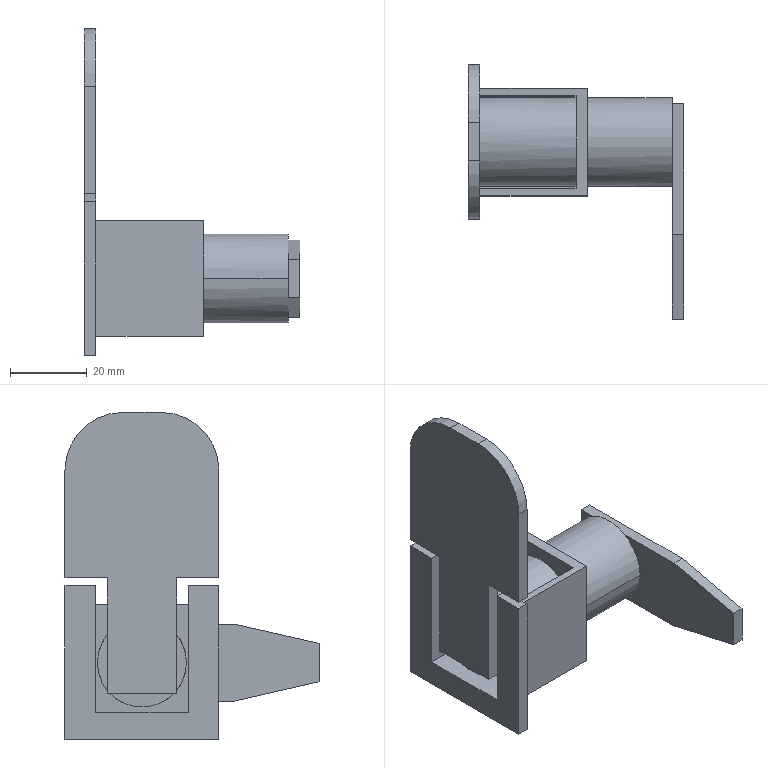Part | NX | features solid 2 | 1 solid | 50 faces | box 56 x 66 x 85 mm | volume 38408 mm3 | plane 44 | cylinder 6 | commonest cylinder face diameters 23.127 x4 30 x2
STEP:
#1=CARTESIAN_POINT('',(-1113.,-1266.5,497.5));
#2=VERTEX_POINT('',#1);
#3=CARTESIAN_POINT('',(-1113.,-1266.5,537.5));
#4=VERTEX_POINT('',#3);
#5=CARTESIAN_POINT('',(-1113.,-1266.5,497.5));
#6=DIRECTION('',(0.,0.,1.));
#7=VECTOR('',#6,1000.);
#8=LINE('',#5,#7);
#9=EDGE_CURVE('',#2,#4,#8,.T.);
#10=ORIENTED_EDGE('',*,*,#9,.T.);
#11=CARTESIAN_POINT('',(-1113.,-1258.5,537.5));
#12=VERTEX_POINT('',#11);
#13=CARTESIAN_POINT('',(-1113.,-1266.5,537.5));
#14=DIRECTION('',(0.,1.,0.));
#15=VECTOR('',#14,1000.);
#16=LINE('',#13,#15);
#17=EDGE_CURVE('',#4,#12,#16,.T.);
#18=ORIENTED_EDGE('',*,*,#17,.T.);
#19=CARTESIAN_POINT('',(-1113.,-1258.5,504.5));
#20=VERTEX_POINT('',#19);
#21=CARTESIAN_POINT('',(-1113.,-1258.5,537.5));
#22=DIRECTION('',(0.,0.,-1.));
#23=VECTOR('',#22,1000.);
#24=LINE('',#21,#23);
#25=EDGE_CURVE('',#12,#20,#24,.T.);
#26=ORIENTED_EDGE('',*,*,#25,.T.);
#27=CARTESIAN_POINT('',(-1113.,-1234.5,504.5));
#28=VERTEX_POINT('',#27);
#29=CARTESIAN_POINT('',(-1113.,-1258.5,504.5));
#30=DIRECTION('',(0.,1.,0.));
#31=VECTOR('',#30,1000.);
#32=LINE('',#29,#31);
#33=EDGE_CURVE('',#20,#28,#32,.T.);
#34=ORIENTED_EDGE('',*,*,#33,.T.);
#35=CARTESIAN_POINT('',(-1113.,-1234.5,537.5));
#36=VERTEX_POINT('',#35);
#37=CARTESIAN_POINT('',(-1113.,-1234.5,504.5));
#38=DIRECTION('',(0.,0.,1.));
#39=VECTOR('',#38,1000.);
#40=LINE('',#37,#39);
#41=EDGE_CURVE('',#28,#36,#40,.T.);
#42=ORIENTED_EDGE('',*,*,#41,.T.);
#43=CARTESIAN_POINT('',(-1113.,-1226.5,537.5));
#44=VERTEX_POINT('',#43);
#45=CARTESIAN_POINT('',(-1113.,-1234.5,537.5));
#46=DIRECTION('',(0.,1.,0.));
#47=VECTOR('',#46,1000.);
#48=LINE('',#45,#47);
#49=EDGE_CURVE('',#36,#44,#48,.T.);
#50=ORIENTED_EDGE('',*,*,#49,.T.);
#51=CARTESIAN_POINT('',(-1113.,-1226.5,497.5));
#52=VERTEX_POINT('',#51);
#53=CARTESIAN_POINT('',(-1113.,-1226.5,537.5));
#54=DIRECTION('',(0.,0.,-1.));
#55=VECTOR('',#54,1000.);
#56=LINE('',#53,#55);
#57=EDGE_CURVE('',#44,#52,#56,.T.);
#58=ORIENTED_EDGE('',*,*,#57,.T.);
#59=CARTESIAN_POINT('',(-1113.,-1226.5,497.5));
#60=DIRECTION('',(0.,-1.,0.));
#61=VECTOR('',#60,1000.);
#62=LINE('',#59,#61);
#63=EDGE_CURVE('',#52,#2,#62,.T.);
#64=ORIENTED_EDGE('',*,*,#63,.T.);
#65=EDGE_LOOP('',(#10,#18,#26,#34,#42,#50,#58,#64));
#66=FACE_BOUND('',#65,.T.);
#67=CARTESIAN_POINT('',(-1113.,-1266.5,537.5));
#68=DIRECTION('',(-1.,0.,0.));
#69=DIRECTION('',(0.,1.,0.));
#70=AXIS2_PLACEMENT_3D('',#67,#68,#69);
#71=PLANE('',#70);
#72=ADVANCED_FACE('',(#66),#71,.T.);
#73=CARTESIAN_POINT('',(-1110.,-1226.5,497.5));
#74=VERTEX_POINT('',#73);
#75=CARTESIAN_POINT('',(-1110.,-1266.5,497.5));
#76=VERTEX_POINT('',#75);
#77=CARTESIAN_POINT('',(-1110.,-1226.5,497.5));
#78=DIRECTION('',(0.,-1.,0.));
#79=VECTOR('',#78,1000.);
#80=LINE('',#77,#79);
#81=EDGE_CURVE('',#74,#76,#80,.T.);
#82=ORIENTED_EDGE('',*,*,#81,.T.);
#83=CARTESIAN_POINT('',(-1113.,-1266.5,497.5));
#84=DIRECTION('',(1.,0.,0.));
#85=VECTOR('',#84,1000.);
#86=LINE('',#83,#85);
#87=EDGE_CURVE('',#2,#76,#86,.T.);
#88=ORIENTED_EDGE('',*,*,#87,.F.);
#89=ORIENTED_EDGE('',*,*,#63,.F.);
#90=CARTESIAN_POINT('',(-1113.,-1226.5,497.5));
#91=DIRECTION('',(1.,0.,0.));
#92=VECTOR('',#91,1000.);
#93=LINE('',#90,#92);
#94=EDGE_CURVE('',#52,#74,#93,.T.);
#95=ORIENTED_EDGE('',*,*,#94,.T.);
#96=EDGE_LOOP('',(#82,#88,#89,#95));
#97=FACE_BOUND('',#96,.T.);
#98=CARTESIAN_POINT('',(-1113.,-1226.5,497.5));
#99=DIRECTION('',(0.,0.,1.));
#100=DIRECTION('',(1.,0.,0.));
#101=AXIS2_PLACEMENT_3D('',#98,#99,#100);
#102=PLANE('',#101);
#103=ADVANCED_FACE('',(#97),#102,.F.);
#104=CARTESIAN_POINT('',(-1110.,-1226.5,537.5));
#105=VERTEX_POINT('',#104);
#106=CARTESIAN_POINT('',(-1110.,-1226.5,537.5));
#107=DIRECTION('',(0.,0.,-1.));
#108=VECTOR('',#107,1000.);
#109=LINE('',#106,#108);
#110=EDGE_CURVE('',#105,#74,#109,.T.);
#111=ORIENTED_EDGE('',*,*,#110,.T.);
#112=ORIENTED_EDGE('',*,*,#94,.F.);
#113=ORIENTED_EDGE('',*,*,#57,.F.);
#114=CARTESIAN_POINT('',(-1113.,-1226.5,537.5));
#115=DIRECTION('',(1.,0.,0.));
#116=VECTOR('',#115,1000.);
#117=LINE('',#114,#116);
#118=EDGE_CURVE('',#44,#105,#117,.T.);
#119=ORIENTED_EDGE('',*,*,#118,.T.);
#120=EDGE_LOOP('',(#111,#112,#113,#119));
#121=FACE_BOUND('',#120,.T.);
#122=CARTESIAN_POINT('',(-1113.,-1226.5,537.5));
#123=DIRECTION('',(0.,-1.,0.));
#124=DIRECTION('',(-1.,0.,0.));
#125=AXIS2_PLACEMENT_3D('',#122,#123,#124);
#126=PLANE('',#125);
#127=ADVANCED_FACE('',(#121),#126,.F.);
#128=CARTESIAN_POINT('',(-1110.,-1234.5,537.5));
#129=VERTEX_POINT('',#128);
#130=CARTESIAN_POINT('',(-1110.,-1234.5,537.5));
#131=DIRECTION('',(0.,1.,0.));
#132=VECTOR('',#131,1000.);
#133=LINE('',#130,#132);
#134=EDGE_CURVE('',#129,#105,#133,.T.);
#135=ORIENTED_EDGE('',*,*,#134,.T.);
#136=ORIENTED_EDGE('',*,*,#118,.F.);
#137=ORIENTED_EDGE('',*,*,#49,.F.);
#138=CARTESIAN_POINT('',(-1113.,-1234.5,537.5));
#139=DIRECTION('',(1.,0.,0.));
#140=VECTOR('',#139,1000.);
#141=LINE('',#138,#140);
#142=EDGE_CURVE('',#36,#129,#141,.T.);
#143=ORIENTED_EDGE('',*,*,#142,.T.);
#144=EDGE_LOOP('',(#135,#136,#137,#143));
#145=FACE_BOUND('',#144,.T.);
#146=CARTESIAN_POINT('',(-1113.,-1234.5,537.5));
#147=DIRECTION('',(0.,0.,-1.));
#148=DIRECTION('',(-1.,0.,0.));
#149=AXIS2_PLACEMENT_3D('',#146,#147,#148);
#150=PLANE('',#149);
#151=ADVANCED_FACE('',(#145),#150,.F.);
#152=CARTESIAN_POINT('',(-1110.,-1266.5,537.5));
#153=VERTEX_POINT('',#152);
#154=CARTESIAN_POINT('',(-1110.,-1258.5,537.5));
#155=VERTEX_POINT('',#154);
#156=CARTESIAN_POINT('',(-1110.,-1266.5,537.5));
#157=DIRECTION('',(0.,1.,0.));
#158=VECTOR('',#157,1000.);
#159=LINE('',#156,#158);
#160=EDGE_CURVE('',#153,#155,#159,.T.);
#161=ORIENTED_EDGE('',*,*,#160,.T.);
#162=CARTESIAN_POINT('',(-1113.,-1258.5,537.5));
#163=DIRECTION('',(1.,0.,0.));
#164=VECTOR('',#163,1000.);
#165=LINE('',#162,#164);
#166=EDGE_CURVE('',#12,#155,#165,.T.);
#167=ORIENTED_EDGE('',*,*,#166,.F.);
#168=ORIENTED_EDGE('',*,*,#17,.F.);
#169=CARTESIAN_POINT('',(-1113.,-1266.5,537.5));
#170=DIRECTION('',(1.,0.,0.));
#171=VECTOR('',#170,1000.);
#172=LINE('',#169,#171);
#173=EDGE_CURVE('',#4,#153,#172,.T.);
#174=ORIENTED_EDGE('',*,*,#173,.T.);
#175=EDGE_LOOP('',(#161,#167,#168,#174));
#176=FACE_BOUND('',#175,.T.);
#177=CARTESIAN_POINT('',(-1113.,-1266.5,537.5));
#178=DIRECTION('',(0.,0.,-1.));
#179=DIRECTION('',(-1.,0.,0.));
#180=AXIS2_PLACEMENT_3D('',#177,#178,#179);
#181=PLANE('',#180);
#182=ADVANCED_FACE('',(#176),#181,.F.);
#183=CARTESIAN_POINT('',(-1110.,-1266.5,497.5));
#184=DIRECTION('',(0.,0.,1.));
#185=VECTOR('',#184,1000.);
#186=LINE('',#183,#185);
#187=EDGE_CURVE('',#76,#153,#186,.T.);
#188=ORIENTED_EDGE('',*,*,#187,.T.);
#189=ORIENTED_EDGE('',*,*,#173,.F.);
#190=ORIENTED_EDGE('',*,*,#9,.F.);
#191=ORIENTED_EDGE('',*,*,#87,.T.);
#192=EDGE_LOOP('',(#188,#189,#190,#191));
#193=FACE_BOUND('',#192,.T.);
#194=CARTESIAN_POINT('',(-1113.,-1266.5,497.5));
#195=DIRECTION('',(0.,1.,0.));
#196=DIRECTION('',(0.,0.,-1.));
#197=AXIS2_PLACEMENT_3D('',#194,#195,#196);
#198=PLANE('',#197);
#199=ADVANCED_FACE('',(#193),#198,.F.);
#200=CARTESIAN_POINT('',(-1110.,-1260.5,502.5));
#201=VERTEX_POINT('',#200);
#202=CARTESIAN_POINT('',(-1110.,-1260.5,532.5));
#203=VERTEX_POINT('',#202);
#204=CARTESIAN_POINT('',(-1110.,-1260.5,502.5));
#205=DIRECTION('',(0.,0.,1.));
#206=VECTOR('',#205,1000.);
#207=LINE('',#204,#206);
#208=EDGE_CURVE('',#201,#203,#207,.T.);
#209=ORIENTED_EDGE('',*,*,#208,.T.);
#210=CARTESIAN_POINT('',(-1110.,-1258.5,532.5));
#211=VERTEX_POINT('',#210);
#212=CARTESIAN_POINT('',(-1110.,-1260.5,532.5));
#213=DIRECTION('',(0.,1.,0.));
#214=VECTOR('',#213,1000.);
#215=LINE('',#212,#214);
#216=EDGE_CURVE('',#203,#211,#215,.T.);
#217=ORIENTED_EDGE('',*,*,#216,.T.);
#218=CARTESIAN_POINT('',(-1110.,-1258.5,537.5));
#219=DIRECTION('',(0.,0.,-1.));
#220=VECTOR('',#219,1000.);
#221=LINE('',#218,#220);
#222=EDGE_CURVE('',#155,#211,#221,.T.);
#223=ORIENTED_EDGE('',*,*,#222,.F.);
#224=ORIENTED_EDGE('',*,*,#160,.F.);
#225=ORIENTED_EDGE('',*,*,#187,.F.);
#226=ORIENTED_EDGE('',*,*,#81,.F.);
#227=ORIENTED_EDGE('',*,*,#110,.F.);
#228=ORIENTED_EDGE('',*,*,#134,.F.);
#229=CARTESIAN_POINT('',(-1110.,-1234.5,532.5));
#230=VERTEX_POINT('',#229);
#231=CARTESIAN_POINT('',(-1110.,-1234.5,504.5));
#232=DIRECTION('',(0.,0.,1.));
#233=VECTOR('',#232,1000.);
#234=LINE('',#231,#233);
#235=EDGE_CURVE('',#230,#129,#234,.T.);
#236=ORIENTED_EDGE('',*,*,#235,.F.);
#237=CARTESIAN_POINT('',(-1110.,-1232.5,532.5));
#238=VERTEX_POINT('',#237);
#239=CARTESIAN_POINT('',(-1110.,-1234.5,532.5));
#240=DIRECTION('',(0.,1.,0.));
#241=VECTOR('',#240,1000.);
#242=LINE('',#239,#241);
#243=EDGE_CURVE('',#230,#238,#242,.T.);
#244=ORIENTED_EDGE('',*,*,#243,.T.);
#245=CARTESIAN_POINT('',(-1110.,-1232.5,502.5));
#246=VERTEX_POINT('',#245);
#247=CARTESIAN_POINT('',(-1110.,-1232.5,532.5));
#248=DIRECTION('',(0.,0.,-1.));
#249=VECTOR('',#248,1000.);
#250=LINE('',#247,#249);
#251=EDGE_CURVE('',#238,#246,#250,.T.);
#252=ORIENTED_EDGE('',*,*,#251,.T.);
#253=CARTESIAN_POINT('',(-1110.,-1232.5,502.5));
#254=DIRECTION('',(0.,-1.,0.));
#255=VECTOR('',#254,1000.);
#256=LINE('',#253,#255);
#257=EDGE_CURVE('',#246,#201,#256,.T.);
#258=ORIENTED_EDGE('',*,*,#257,.T.);
#259=EDGE_LOOP('',(#209,#217,#223,#224,#225,#226,#227,#228,#236,#244,#252,#258));
#260=FACE_BOUND('',#259,.T.);
#261=CARTESIAN_POINT('',(-1110.,-1266.5,537.5));
#262=DIRECTION('',(-1.,0.,0.));
#263=DIRECTION('',(0.,1.,0.));
#264=AXIS2_PLACEMENT_3D('',#261,#262,#263);
#265=PLANE('',#264);
#266=ADVANCED_FACE('',(#260),#265,.F.);
#267=CARTESIAN_POINT('',(-1110.,-1238.151,509.5));
#268=VERTEX_POINT('',#267);
#269=CARTESIAN_POINT('',(-1110.,-1237.5,510.24));
#270=VERTEX_POINT('',#269);
#271=CARTESIAN_POINT('',(-1110.,-1246.5,517.5));
#272=DIRECTION('',(1.,0.,0.));
#273=DIRECTION('',(0.,1.,0.));
#274=AXIS2_PLACEMENT_3D('',#271,#272,#273);
#275=CIRCLE('',#274,11.563);
#276=EDGE_CURVE('',#268,#270,#275,.T.);
#277=ORIENTED_EDGE('',*,*,#276,.F.);
#278=CARTESIAN_POINT('',(-1110.,-1237.5,509.5));
#279=VERTEX_POINT('',#278);
#280=CARTESIAN_POINT('',(-1110.,-1237.5,509.5));
#281=DIRECTION('',(0.,-1.,0.));
#282=VECTOR('',#281,1000.);
#283=LINE('',#280,#282);
#284=EDGE_CURVE('',#279,#268,#283,.T.);
#285=ORIENTED_EDGE('',*,*,#284,.F.);
#286=CARTESIAN_POINT('',(-1110.,-1237.5,539.5));
#287=DIRECTION('',(0.,0.,-1.));
#288=VECTOR('',#287,1000.);
#289=LINE('',#286,#288);
#290=EDGE_CURVE('',#270,#279,#289,.T.);
#291=ORIENTED_EDGE('',*,*,#290,.F.);
#292=EDGE_LOOP('',(#277,#285,#291));
#293=FACE_BOUND('',#292,.T.);
#294=CARTESIAN_POINT('',(-1110.,-1251.5,567.5));
#295=DIRECTION('',(-1.,0.,0.));
#296=DIRECTION('',(0.,1.,0.));
#297=AXIS2_PLACEMENT_3D('',#294,#295,#296);
#298=PLANE('',#297);
#299=ADVANCED_FACE('',(#293),#298,.F.);
#300=CARTESIAN_POINT('',(-1113.,-1226.5,539.5));
#301=VERTEX_POINT('',#300);
#302=CARTESIAN_POINT('',(-1113.,-1237.5,539.5));
#303=VERTEX_POINT('',#302);
#304=CARTESIAN_POINT('',(-1113.,-1226.5,539.5));
#305=DIRECTION('',(0.,-1.,0.));
#306=VECTOR('',#305,1000.);
#307=LINE('',#304,#306);
#308=EDGE_CURVE('',#301,#303,#307,.T.);
#309=ORIENTED_EDGE('',*,*,#308,.T.);
#310=CARTESIAN_POINT('',(-1113.,-1237.5,509.5));
#311=VERTEX_POINT('',#310);
#312=CARTESIAN_POINT('',(-1113.,-1237.5,539.5));
#313=DIRECTION('',(0.,0.,-1.));
#314=VECTOR('',#313,1000.);
#315=LINE('',#312,#314);
#316=EDGE_CURVE('',#303,#311,#315,.T.);
#317=ORIENTED_EDGE('',*,*,#316,.T.);
#318=CARTESIAN_POINT('',(-1113.,-1255.5,509.5));
#319=VERTEX_POINT('',#318);
#320=CARTESIAN_POINT('',(-1113.,-1237.5,509.5));
#321=DIRECTION('',(0.,-1.,0.));
#322=VECTOR('',#321,1000.);
#323=LINE('',#320,#322);
#324=EDGE_CURVE('',#311,#319,#323,.T.);
#325=ORIENTED_EDGE('',*,*,#324,.T.);
#326=CARTESIAN_POINT('',(-1113.,-1255.5,539.5));
#327=VERTEX_POINT('',#326);
#328=CARTESIAN_POINT('',(-1113.,-1255.5,509.5));
#329=DIRECTION('',(0.,0.,1.));
#330=VECTOR('',#329,1000.);
#331=LINE('',#328,#330);
#332=EDGE_CURVE('',#319,#327,#331,.T.);
#333=ORIENTED_EDGE('',*,*,#332,.T.);
#334=CARTESIAN_POINT('',(-1113.,-1266.5,539.5));
#335=VERTEX_POINT('',#334);
#336=CARTESIAN_POINT('',(-1113.,-1255.5,539.5));
#337=DIRECTION('',(0.,-1.,0.));
#338=VECTOR('',#337,1000.);
#339=LINE('',#336,#338);
#340=EDGE_CURVE('',#327,#335,#339,.T.);
#341=ORIENTED_EDGE('',*,*,#340,.T.);
#342=CARTESIAN_POINT('',(-1113.,-1266.5,567.5));
#343=VERTEX_POINT('',#342);
#344=CARTESIAN_POINT('',(-1113.,-1266.5,539.5));
#345=DIRECTION('',(0.,0.,1.));
#346=VECTOR('',#345,1000.);
#347=LINE('',#344,#346);
#348=EDGE_CURVE('',#335,#343,#347,.T.);
#349=ORIENTED_EDGE('',*,*,#348,.T.);
#350=CARTESIAN_POINT('',(-1113.,-1251.5,582.5));
#351=VERTEX_POINT('',#350);
#352=CARTESIAN_POINT('',(-1113.,-1251.5,567.5));
#353=DIRECTION('',(-1.,0.,0.));
#354=DIRECTION('',(0.,1.,0.));
#355=AXIS2_PLACEMENT_3D('',#352,#353,#354);
#356=CIRCLE('',#355,15.);
#357=EDGE_CURVE('',#343,#351,#356,.T.);
#358=ORIENTED_EDGE('',*,*,#357,.T.);
#359=CARTESIAN_POINT('',(-1113.,-1241.5,582.5));
#360=VERTEX_POINT('',#359);
#361=CARTESIAN_POINT('',(-1113.,-1251.5,582.5));
#362=DIRECTION('',(0.,1.,0.));
#363=VECTOR('',#362,1000.);
#364=LINE('',#361,#363);
#365=EDGE_CURVE('',#351,#360,#364,.T.);
#366=ORIENTED_EDGE('',*,*,#365,.T.);
#367=CARTESIAN_POINT('',(-1113.,-1226.5,567.5));
#368=VERTEX_POINT('',#367);
#369=CARTESIAN_POINT('',(-1113.,-1241.5,567.5));
#370=DIRECTION('',(-1.,0.,0.));
#371=DIRECTION('',(0.,-1.,0.));
#372=AXIS2_PLACEMENT_3D('',#369,#370,#371);
#373=CIRCLE('',#372,15.);
#374=EDGE_CURVE('',#360,#368,#373,.T.);
#375=ORIENTED_EDGE('',*,*,#374,.T.);
#376=CARTESIAN_POINT('',(-1113.,-1226.5,567.5));
#377=DIRECTION('',(0.,0.,-1.));
#378=VECTOR('',#377,1000.);
#379=LINE('',#376,#378);
#380=EDGE_CURVE('',#368,#301,#379,.T.);
#381=ORIENTED_EDGE('',*,*,#380,.T.);
#382=EDGE_LOOP('',(#309,#317,#325,#333,#341,#349,#358,#366,#375,#381));
#383=FACE_BOUND('',#382,.T.);
#384=CARTESIAN_POINT('',(-1113.,-1251.5,567.5));
#385=DIRECTION('',(-1.,0.,0.));
#386=DIRECTION('',(0.,1.,0.));
#387=AXIS2_PLACEMENT_3D('',#384,#385,#386);
#388=PLANE('',#387);
#389=ADVANCED_FACE('',(#383),#388,.T.);
#390=CARTESIAN_POINT('',(-1110.,-1226.5,567.5));
#391=VERTEX_POINT('',#390);
#392=CARTESIAN_POINT('',(-1110.,-1226.5,539.5));
#393=VERTEX_POINT('',#392);
#394=CARTESIAN_POINT('',(-1110.,-1226.5,567.5));
#395=DIRECTION('',(0.,0.,-1.));
#396=VECTOR('',#395,1000.);
#397=LINE('',#394,#396);
#398=EDGE_CURVE('',#391,#393,#397,.T.);
#399=ORIENTED_EDGE('',*,*,#398,.T.);
#400=CARTESIAN_POINT('',(-1113.,-1226.5,539.5));
#401=DIRECTION('',(1.,0.,0.));
#402=VECTOR('',#401,1000.);
#403=LINE('',#400,#402);
#404=EDGE_CURVE('',#301,#393,#403,.T.);
#405=ORIENTED_EDGE('',*,*,#404,.F.);
#406=ORIENTED_EDGE('',*,*,#380,.F.);
#407=CARTESIAN_POINT('',(-1113.,-1226.5,567.5));
#408=DIRECTION('',(1.,0.,0.));
#409=VECTOR('',#408,1000.);
#410=LINE('',#407,#409);
#411=EDGE_CURVE('',#368,#391,#410,.T.);
#412=ORIENTED_EDGE('',*,*,#411,.T.);
#413=EDGE_LOOP('',(#399,#405,#406,#412));
#414=FACE_BOUND('',#413,.T.);
#415=CARTESIAN_POINT('',(-1113.,-1226.5,567.5));
#416=DIRECTION('',(0.,-1.,0.));
#417=DIRECTION('',(-1.,0.,0.));
#418=AXIS2_PLACEMENT_3D('',#415,#416,#417);
#419=PLANE('',#418);
#420=ADVANCED_FACE('',(#414),#419,.F.);
#421=CARTESIAN_POINT('',(-1110.,-1241.5,582.5));
#422=VERTEX_POINT('',#421);
#423=CARTESIAN_POINT('',(-1110.,-1241.5,567.5));
#424=DIRECTION('',(-1.,0.,0.));
#425=DIRECTION('',(0.,-1.,0.));
#426=AXIS2_PLACEMENT_3D('',#423,#424,#425);
#427=CIRCLE('',#426,15.);
#428=EDGE_CURVE('',#422,#391,#427,.T.);
#429=ORIENTED_EDGE('',*,*,#428,.T.);
#430=ORIENTED_EDGE('',*,*,#411,.F.);
#431=ORIENTED_EDGE('',*,*,#374,.F.);
#432=CARTESIAN_POINT('',(-1113.,-1241.5,582.5));
#433=DIRECTION('',(1.,0.,0.));
#434=VECTOR('',#433,1000.);
#435=LINE('',#432,#434);
#436=EDGE_CURVE('',#360,#422,#435,.T.);
#437=ORIENTED_EDGE('',*,*,#436,.T.);
#438=EDGE_LOOP('',(#429,#430,#431,#437));
#439=FACE_BOUND('',#438,.T.);
#440=CARTESIAN_POINT('',(-1113.,-1241.5,567.5));
#441=DIRECTION('',(1.,0.,0.));
#442=DIRECTION('',(0.,-1.,0.));
#443=AXIS2_PLACEMENT_3D('',#440,#441,#442);
#444=CYLINDRICAL_SURFACE('',#443,15.);
#445=ADVANCED_FACE('',(#439),#444,.T.);
#446=CARTESIAN_POINT('',(-1110.,-1251.5,582.5));
#447=VERTEX_POINT('',#446);
#448=CARTESIAN_POINT('',(-1110.,-1251.5,582.5));
#449=DIRECTION('',(0.,1.,0.));
#450=VECTOR('',#449,1000.);
#451=LINE('',#448,#450);
#452=EDGE_CURVE('',#447,#422,#451,.T.);
#453=ORIENTED_EDGE('',*,*,#452,.T.);
#454=ORIENTED_EDGE('',*,*,#436,.F.);
#455=ORIENTED_EDGE('',*,*,#365,.F.);
#456=CARTESIAN_POINT('',(-1113.,-1251.5,582.5));
#457=DIRECTION('',(1.,0.,0.));
#458=VECTOR('',#457,1000.);
#459=LINE('',#456,#458);
#460=EDGE_CURVE('',#351,#447,#459,.T.);
#461=ORIENTED_EDGE('',*,*,#460,.T.);
#462=EDGE_LOOP('',(#453,#454,#455,#461));
#463=FACE_BOUND('',#462,.T.);
#464=CARTESIAN_POINT('',(-1113.,-1251.5,582.5));
#465=DIRECTION('',(0.,0.,-1.));
#466=DIRECTION('',(-1.,0.,0.));
#467=AXIS2_PLACEMENT_3D('',#464,#465,#466);
#468=PLANE('',#467);
#469=ADVANCED_FACE('',(#463),#468,.F.);
#470=CARTESIAN_POINT('',(-1110.,-1266.5,567.5));
#471=VERTEX_POINT('',#470);
#472=CARTESIAN_POINT('',(-1110.,-1251.5,567.5));
#473=DIRECTION('',(-1.,0.,0.));
#474=DIRECTION('',(0.,1.,0.));
#475=AXIS2_PLACEMENT_3D('',#472,#473,#474);
#476=CIRCLE('',#475,15.);
#477=EDGE_CURVE('',#471,#447,#476,.T.);
#478=ORIENTED_EDGE('',*,*,#477,.T.);
#479=ORIENTED_EDGE('',*,*,#460,.F.);
#480=ORIENTED_EDGE('',*,*,#357,.F.);
#481=CARTESIAN_POINT('',(-1113.,-1266.5,567.5));
#482=DIRECTION('',(1.,0.,0.));
#483=VECTOR('',#482,1000.);
#484=LINE('',#481,#483);
#485=EDGE_CURVE('',#343,#471,#484,.T.);
#486=ORIENTED_EDGE('',*,*,#485,.T.);
#487=EDGE_LOOP('',(#478,#479,#480,#486));
#488=FACE_BOUND('',#487,.T.);
#489=CARTESIAN_POINT('',(-1113.,-1251.5,567.5));
#490=DIRECTION('',(1.,0.,0.));
#491=DIRECTION('',(0.,-1.,0.));
#492=AXIS2_PLACEMENT_3D('',#489,#490,#491);
#493=CYLINDRICAL_SURFACE('',#492,15.);
#494=ADVANCED_FACE('',(#488),#493,.T.);
#495=CARTESIAN_POINT('',(-1110.,-1266.5,539.5));
#496=VERTEX_POINT('',#495);
#497=CARTESIAN_POINT('',(-1110.,-1266.5,539.5));
#498=DIRECTION('',(0.,0.,1.));
#499=VECTOR('',#498,1000.);
#500=LINE('',#497,#499);
#501=EDGE_CURVE('',#496,#471,#500,.T.);
#502=ORIENTED_EDGE('',*,*,#501,.T.);
#503=ORIENTED_EDGE('',*,*,#485,.F.);
#504=ORIENTED_EDGE('',*,*,#348,.F.);
#505=CARTESIAN_POINT('',(-1113.,-1266.5,539.5));
#506=DIRECTION('',(1.,0.,0.));
#507=VECTOR('',#506,1000.);
#508=LINE('',#505,#507);
#509=EDGE_CURVE('',#335,#496,#508,.T.);
#510=ORIENTED_EDGE('',*,*,#509,.T.);
#511=EDGE_LOOP('',(#502,#503,#504,#510));
#512=FACE_BOUND('',#511,.T.);
#513=CARTESIAN_POINT('',(-1113.,-1266.5,539.5));
#514=DIRECTION('',(0.,1.,0.));
#515=DIRECTION('',(0.,0.,-1.));
#516=AXIS2_PLACEMENT_3D('',#513,#514,#515);
#517=PLANE('',#516);
#518=ADVANCED_FACE('',(#512),#517,.F.);
#519=CARTESIAN_POINT('',(-1110.,-1255.5,539.5));
#520=VERTEX_POINT('',#519);
#521=CARTESIAN_POINT('',(-1110.,-1255.5,539.5));
#522=DIRECTION('',(0.,-1.,0.));
#523=VECTOR('',#522,1000.);
#524=LINE('',#521,#523);
#525=EDGE_CURVE('',#520,#496,#524,.T.);
#526=ORIENTED_EDGE('',*,*,#525,.T.);
#527=ORIENTED_EDGE('',*,*,#509,.F.);
#528=ORIENTED_EDGE('',*,*,#340,.F.);
#529=CARTESIAN_POINT('',(-1113.,-1255.5,539.5));
#530=DIRECTION('',(1.,0.,0.));
#531=VECTOR('',#530,1000.);
#532=LINE('',#529,#531);
#533=EDGE_CURVE('',#327,#520,#532,.T.);
#534=ORIENTED_EDGE('',*,*,#533,.T.);
#535=EDGE_LOOP('',(#526,#527,#528,#534));
#536=FACE_BOUND('',#535,.T.);
#537=CARTESIAN_POINT('',(-1113.,-1255.5,539.5));
#538=DIRECTION('',(0.,0.,1.));
#539=DIRECTION('',(1.,0.,0.));
#540=AXIS2_PLACEMENT_3D('',#537,#538,#539);
#541=PLANE('',#540);
#542=ADVANCED_FACE('',(#536),#541,.F.);
#543=CARTESIAN_POINT('',(-1110.,-1255.5,509.5));
#544=VERTEX_POINT('',#543);
#545=CARTESIAN_POINT('',(-1110.,-1255.5,510.24));
#546=VERTEX_POINT('',#545);
#547=CARTESIAN_POINT('',(-1110.,-1255.5,509.5));
#548=DIRECTION('',(0.,0.,1.));
#549=VECTOR('',#548,1000.);
#550=LINE('',#547,#549);
#551=EDGE_CURVE('',#544,#546,#550,.T.);
#552=ORIENTED_EDGE('',*,*,#551,.T.);
#553=CARTESIAN_POINT('',(-1110.,-1255.5,524.76));
#554=VERTEX_POINT('',#553);
#555=CARTESIAN_POINT('',(-1110.,-1255.5,509.5));
#556=DIRECTION('',(0.,0.,1.));
#557=VECTOR('',#556,1000.);
#558=LINE('',#555,#557);
#559=EDGE_CURVE('',#546,#554,#558,.T.);
#560=ORIENTED_EDGE('',*,*,#559,.T.);
#561=CARTESIAN_POINT('',(-1110.,-1255.5,509.5));
#562=DIRECTION('',(0.,0.,1.));
#563=VECTOR('',#562,1000.);
#564=LINE('',#561,#563);
#565=EDGE_CURVE('',#554,#520,#564,.T.);
#566=ORIENTED_EDGE('',*,*,#565,.T.);
#567=ORIENTED_EDGE('',*,*,#533,.F.);
#568=ORIENTED_EDGE('',*,*,#332,.F.);
#569=CARTESIAN_POINT('',(-1113.,-1255.5,509.5));
#570=DIRECTION('',(1.,0.,0.));
#571=VECTOR('',#570,1000.);
#572=LINE('',#569,#571);
#573=EDGE_CURVE('',#319,#544,#572,.T.);
#574=ORIENTED_EDGE('',*,*,#573,.T.);
#575=EDGE_LOOP('',(#552,#560,#566,#567,#568,#574));
#576=FACE_BOUND('',#575,.T.);
#577=CARTESIAN_POINT('',(-1113.,-1255.5,509.5));
#578=DIRECTION('',(0.,1.,0.));
#579=DIRECTION('',(0.,0.,-1.));
#580=AXIS2_PLACEMENT_3D('',#577,#578,#579);
#581=PLANE('',#580);
#582=ADVANCED_FACE('',(#576),#581,.F.);
#583=ORIENTED_EDGE('',*,*,#284,.T.);
#584=CARTESIAN_POINT('',(-1110.,-1254.849,509.5));
#585=VERTEX_POINT('',#584);
#586=CARTESIAN_POINT('',(-1110.,-1237.5,509.5));
#587=DIRECTION('',(0.,-1.,0.));
#588=VECTOR('',#587,1000.);
#589=LINE('',#586,#588);
#590=EDGE_CURVE('',#268,#585,#589,.T.);
#591=ORIENTED_EDGE('',*,*,#590,.T.);
#592=CARTESIAN_POINT('',(-1110.,-1237.5,509.5));
#593=DIRECTION('',(0.,-1.,0.));
#594=VECTOR('',#593,1000.);
#595=LINE('',#592,#594);
#596=EDGE_CURVE('',#585,#544,#595,.T.);
#597=ORIENTED_EDGE('',*,*,#596,.T.);
#598=ORIENTED_EDGE('',*,*,#573,.F.);
#599=ORIENTED_EDGE('',*,*,#324,.F.);
#600=CARTESIAN_POINT('',(-1113.,-1237.5,509.5));
#601=DIRECTION('',(1.,0.,0.));
#602=VECTOR('',#601,1000.);
#603=LINE('',#600,#602);
#604=EDGE_CURVE('',#311,#279,#603,.T.);
#605=ORIENTED_EDGE('',*,*,#604,.T.);
#606=EDGE_LOOP('',(#583,#591,#597,#598,#599,#605));
#607=FACE_BOUND('',#606,.T.);
#608=CARTESIAN_POINT('',(-1113.,-1237.5,509.5));
#609=DIRECTION('',(0.,0.,1.));
#610=DIRECTION('',(1.,0.,0.));
#611=AXIS2_PLACEMENT_3D('',#608,#609,#610);
#612=PLANE('',#611);
#613=ADVANCED_FACE('',(#607),#612,.F.);
#614=CARTESIAN_POINT('',(-1110.,-1237.5,539.5));
#615=VERTEX_POINT('',#614);
#616=CARTESIAN_POINT('',(-1110.,-1237.5,524.76));
#617=VERTEX_POINT('',#616);
#618=CARTESIAN_POINT('',(-1110.,-1237.5,539.5));
#619=DIRECTION('',(0.,0.,-1.));
#620=VECTOR('',#619,1000.);
#621=LINE('',#618,#620);
#622=EDGE_CURVE('',#615,#617,#621,.T.);
#623=ORIENTED_EDGE('',*,*,#622,.T.);
#624=CARTESIAN_POINT('',(-1110.,-1237.5,539.5));
#625=DIRECTION('',(0.,0.,-1.));
#626=VECTOR('',#625,1000.);
#627=LINE('',#624,#626);
#628=EDGE_CURVE('',#617,#270,#627,.T.);
#629=ORIENTED_EDGE('',*,*,#628,.T.);
#630=ORIENTED_EDGE('',*,*,#290,.T.);
#631=ORIENTED_EDGE('',*,*,#604,.F.);
#632=ORIENTED_EDGE('',*,*,#316,.F.);
#633=CARTESIAN_POINT('',(-1113.,-1237.5,539.5));
#634=DIRECTION('',(1.,0.,0.));
#635=VECTOR('',#634,1000.);
#636=LINE('',#633,#635);
#637=EDGE_CURVE('',#303,#615,#636,.T.);
#638=ORIENTED_EDGE('',*,*,#637,.T.);
#639=EDGE_LOOP('',(#623,#629,#630,#631,#632,#638));
#640=FACE_BOUND('',#639,.T.);
#641=CARTESIAN_POINT('',(-1113.,-1237.5,539.5));
#642=DIRECTION('',(0.,-1.,0.));
#643=DIRECTION('',(-1.,0.,0.));
#644=AXIS2_PLACEMENT_3D('',#641,#642,#643);
#645=PLANE('',#644);
#646=ADVANCED_FACE('',(#640),#645,.F.);
#647=CARTESIAN_POINT('',(-1110.,-1226.5,539.5));
#648=DIRECTION('',(0.,-1.,0.));
#649=VECTOR('',#648,1000.);
#650=LINE('',#647,#649);
#651=EDGE_CURVE('',#393,#615,#650,.T.);
#652=ORIENTED_EDGE('',*,*,#651,.T.);
#653=ORIENTED_EDGE('',*,*,#637,.F.);
#654=ORIENTED_EDGE('',*,*,#308,.F.);
#655=ORIENTED_EDGE('',*,*,#404,.T.);
#656=EDGE_LOOP('',(#652,#653,#654,#655));
#657=FACE_BOUND('',#656,.T.);
#658=CARTESIAN_POINT('',(-1113.,-1226.5,539.5));
#659=DIRECTION('',(0.,0.,1.));
#660=DIRECTION('',(1.,0.,0.));
#661=AXIS2_PLACEMENT_3D('',#658,#659,#660);
#662=PLANE('',#661);
#663=ADVANCED_FACE('',(#657),#662,.F.);
#664=CARTESIAN_POINT('',(-1110.,-1246.5,517.5));
#665=DIRECTION('',(1.,0.,0.));
#666=DIRECTION('',(0.,1.,0.));
#667=AXIS2_PLACEMENT_3D('',#664,#665,#666);
#668=CIRCLE('',#667,11.563);
#669=EDGE_CURVE('',#546,#585,#668,.T.);
#670=ORIENTED_EDGE('',*,*,#669,.F.);
#671=ORIENTED_EDGE('',*,*,#551,.F.);
#672=ORIENTED_EDGE('',*,*,#596,.F.);
#673=EDGE_LOOP('',(#670,#671,#672));
#674=FACE_BOUND('',#673,.T.);
#675=CARTESIAN_POINT('',(-1110.,-1251.5,567.5));
#676=DIRECTION('',(-1.,0.,0.));
#677=DIRECTION('',(0.,1.,0.));
#678=AXIS2_PLACEMENT_3D('',#675,#676,#677);
#679=PLANE('',#678);
#680=ADVANCED_FACE('',(#674),#679,.F.);
#681=CARTESIAN_POINT('',(-1110.,-1246.5,517.5));
#682=DIRECTION('',(1.,0.,0.));
#683=DIRECTION('',(0.,1.,0.));
#684=AXIS2_PLACEMENT_3D('',#681,#682,#683);
#685=CIRCLE('',#684,11.563);
#686=EDGE_CURVE('',#617,#554,#685,.T.);
#687=ORIENTED_EDGE('',*,*,#686,.F.);
#688=ORIENTED_EDGE('',*,*,#622,.F.);
#689=ORIENTED_EDGE('',*,*,#651,.F.);
#690=ORIENTED_EDGE('',*,*,#398,.F.);
#691=ORIENTED_EDGE('',*,*,#428,.F.);
#692=ORIENTED_EDGE('',*,*,#452,.F.);
#693=ORIENTED_EDGE('',*,*,#477,.F.);
#694=ORIENTED_EDGE('',*,*,#501,.F.);
#695=ORIENTED_EDGE('',*,*,#525,.F.);
#696=ORIENTED_EDGE('',*,*,#565,.F.);
#697=EDGE_LOOP('',(#687,#688,#689,#690,#691,#692,#693,#694,#695,#696));
#698=FACE_BOUND('',#697,.T.);
#699=CARTESIAN_POINT('',(-1110.,-1251.5,567.5));
#700=DIRECTION('',(-1.,0.,0.));
#701=DIRECTION('',(0.,1.,0.));
#702=AXIS2_PLACEMENT_3D('',#699,#700,#701);
#703=PLANE('',#702);
#704=ADVANCED_FACE('',(#698),#703,.F.);
#705=CARTESIAN_POINT('',(-1057.,-1270.5,507.5));
#706=VERTEX_POINT('',#705);
#707=CARTESIAN_POINT('',(-1057.,-1292.5,512.5));
#708=VERTEX_POINT('',#707);
#709=CARTESIAN_POINT('',(-1057.,-1270.5,507.5));
#710=DIRECTION('',(0.,-0.9751,0.2216));
#711=VECTOR('',#710,1000.);
#712=LINE('',#709,#711);
#713=EDGE_CURVE('',#706,#708,#712,.T.);
#714=ORIENTED_EDGE('',*,*,#713,.F.);
#715=CARTESIAN_POINT('',(-1057.,-1236.5,507.5));
#716=VERTEX_POINT('',#715);
#717=CARTESIAN_POINT('',(-1057.,-1236.5,507.5));
#718=DIRECTION('',(0.,-1.,0.));
#719=VECTOR('',#718,1000.);
#720=LINE('',#717,#719);
#721=EDGE_CURVE('',#716,#706,#720,.T.);
#722=ORIENTED_EDGE('',*,*,#721,.F.);
#723=CARTESIAN_POINT('',(-1057.,-1236.5,527.5));
#724=VERTEX_POINT('',#723);
#725=CARTESIAN_POINT('',(-1057.,-1236.5,527.5));
#726=DIRECTION('',(0.,0.,-1.));
#727=VECTOR('',#726,1000.);
#728=LINE('',#725,#727);
#729=EDGE_CURVE('',#724,#716,#728,.T.);
#730=ORIENTED_EDGE('',*,*,#729,.F.);
#731=CARTESIAN_POINT('',(-1057.,-1270.5,527.5));
#732=VERTEX_POINT('',#731);
#733=CARTESIAN_POINT('',(-1057.,-1270.5,527.5));
#734=DIRECTION('',(0.,1.,0.));
#735=VECTOR('',#734,1000.);
#736=LINE('',#733,#735);
#737=EDGE_CURVE('',#732,#724,#736,.T.);
#738=ORIENTED_EDGE('',*,*,#737,.F.);
#739=CARTESIAN_POINT('',(-1057.,-1292.5,522.5));
#740=VERTEX_POINT('',#739);
#741=CARTESIAN_POINT('',(-1057.,-1292.5,522.5));
#742=DIRECTION('',(0.,0.9751,0.2216));
#743=VECTOR('',#742,1000.);
#744=LINE('',#741,#743);
#745=EDGE_CURVE('',#740,#732,#744,.T.);
#746=ORIENTED_EDGE('',*,*,#745,.F.);
#747=CARTESIAN_POINT('',(-1057.,-1292.5,512.5));
#748=DIRECTION('',(0.,0.,1.));
#749=VECTOR('',#748,1000.);
#750=LINE('',#747,#749);
#751=EDGE_CURVE('',#708,#740,#750,.T.);
#752=ORIENTED_EDGE('',*,*,#751,.F.);
#753=EDGE_LOOP('',(#714,#722,#730,#738,#746,#752));
#754=FACE_BOUND('',#753,.T.);
#755=CARTESIAN_POINT('',(-1057.,-1292.5,512.5));
#756=DIRECTION('',(-1.,0.,0.));
#757=DIRECTION('',(0.,1.,0.));
#758=AXIS2_PLACEMENT_3D('',#755,#756,#757);
#759=PLANE('',#758);
#760=ADVANCED_FACE('',(#754),#759,.F.);
#761=CARTESIAN_POINT('',(-1060.,-1236.5,507.5));
#762=VERTEX_POINT('',#761);
#763=CARTESIAN_POINT('',(-1060.,-1240.694,507.5));
#764=VERTEX_POINT('',#763);
#765=CARTESIAN_POINT('',(-1060.,-1236.5,507.5));
#766=DIRECTION('',(0.,-1.,0.));
#767=VECTOR('',#766,1000.);
#768=LINE('',#765,#767);
#769=EDGE_CURVE('',#762,#764,#768,.T.);
#770=ORIENTED_EDGE('',*,*,#769,.F.);
#771=CARTESIAN_POINT('',(-1057.,-1236.5,507.5));
#772=DIRECTION('',(-1.,0.,0.));
#773=VECTOR('',#772,1000.);
#774=LINE('',#771,#773);
#775=EDGE_CURVE('',#716,#762,#774,.T.);
#776=ORIENTED_EDGE('',*,*,#775,.F.);
#777=ORIENTED_EDGE('',*,*,#721,.T.);
#778=CARTESIAN_POINT('',(-1060.,-1270.5,507.5));
#779=VERTEX_POINT('',#778);
#780=CARTESIAN_POINT('',(-1057.,-1270.5,507.5));
#781=DIRECTION('',(-1.,0.,0.));
#782=VECTOR('',#781,1000.);
#783=LINE('',#780,#782);
#784=EDGE_CURVE('',#706,#779,#783,.T.);
#785=ORIENTED_EDGE('',*,*,#784,.T.);
#786=CARTESIAN_POINT('',(-1060.,-1252.306,507.5));
#787=VERTEX_POINT('',#786);
#788=CARTESIAN_POINT('',(-1060.,-1236.5,507.5));
#789=DIRECTION('',(0.,-1.,0.));
#790=VECTOR('',#789,1000.);
#791=LINE('',#788,#790);
#792=EDGE_CURVE('',#787,#779,#791,.T.);
#793=ORIENTED_EDGE('',*,*,#792,.F.);
#794=CARTESIAN_POINT('',(-1060.,-1236.5,507.5));
#795=DIRECTION('',(0.,-1.,0.));
#796=VECTOR('',#795,1000.);
#797=LINE('',#794,#796);
#798=EDGE_CURVE('',#764,#787,#797,.T.);
#799=ORIENTED_EDGE('',*,*,#798,.F.);
#800=EDGE_LOOP('',(#770,#776,#777,#785,#793,#799));
#801=FACE_BOUND('',#800,.T.);
#802=CARTESIAN_POINT('',(-1057.,-1236.5,507.5));
#803=DIRECTION('',(0.,0.,-1.));
#804=DIRECTION('',(-1.,0.,0.));
#805=AXIS2_PLACEMENT_3D('',#802,#803,#804);
#806=PLANE('',#805);
#807=ADVANCED_FACE('',(#801),#806,.T.);
#808=CARTESIAN_POINT('',(-1060.,-1236.5,527.5));
#809=VERTEX_POINT('',#808);
#810=CARTESIAN_POINT('',(-1060.,-1236.5,523.306));
#811=VERTEX_POINT('',#810);
#812=CARTESIAN_POINT('',(-1060.,-1236.5,527.5));
#813=DIRECTION('',(0.,0.,-1.));
#814=VECTOR('',#813,1000.);
#815=LINE('',#812,#814);
#816=EDGE_CURVE('',#809,#811,#815,.T.);
#817=ORIENTED_EDGE('',*,*,#816,.F.);
#818=CARTESIAN_POINT('',(-1057.,-1236.5,527.5));
#819=DIRECTION('',(-1.,0.,0.));
#820=VECTOR('',#819,1000.);
#821=LINE('',#818,#820);
#822=EDGE_CURVE('',#724,#809,#821,.T.);
#823=ORIENTED_EDGE('',*,*,#822,.F.);
#824=ORIENTED_EDGE('',*,*,#729,.T.);
#825=ORIENTED_EDGE('',*,*,#775,.T.);
#826=CARTESIAN_POINT('',(-1060.,-1236.5,511.694));
#827=VERTEX_POINT('',#826);
#828=CARTESIAN_POINT('',(-1060.,-1236.5,527.5));
#829=DIRECTION('',(0.,0.,-1.));
#830=VECTOR('',#829,1000.);
#831=LINE('',#828,#830);
#832=EDGE_CURVE('',#827,#762,#831,.T.);
#833=ORIENTED_EDGE('',*,*,#832,.F.);
#834=CARTESIAN_POINT('',(-1060.,-1236.5,527.5));
#835=DIRECTION('',(0.,0.,-1.));
#836=VECTOR('',#835,1000.);
#837=LINE('',#834,#836);
#838=EDGE_CURVE('',#811,#827,#837,.T.);
#839=ORIENTED_EDGE('',*,*,#838,.F.);
#840=EDGE_LOOP('',(#817,#823,#824,#825,#833,#839));
#841=FACE_BOUND('',#840,.T.);
#842=CARTESIAN_POINT('',(-1057.,-1236.5,527.5));
#843=DIRECTION('',(0.,1.,0.));
#844=DIRECTION('',(0.,0.,-1.));
#845=AXIS2_PLACEMENT_3D('',#842,#843,#844);
#846=PLANE('',#845);
#847=ADVANCED_FACE('',(#841),#846,.T.);
#848=CARTESIAN_POINT('',(-1060.,-1270.5,527.5));
#849=VERTEX_POINT('',#848);
#850=CARTESIAN_POINT('',(-1060.,-1252.306,527.5));
#851=VERTEX_POINT('',#850);
#852=CARTESIAN_POINT('',(-1060.,-1270.5,527.5));
#853=DIRECTION('',(0.,1.,0.));
#854=VECTOR('',#853,1000.);
#855=LINE('',#852,#854);
#856=EDGE_CURVE('',#849,#851,#855,.T.);
#857=ORIENTED_EDGE('',*,*,#856,.F.);
#858=CARTESIAN_POINT('',(-1057.,-1270.5,527.5));
#859=DIRECTION('',(-1.,0.,0.));
#860=VECTOR('',#859,1000.);
#861=LINE('',#858,#860);
#862=EDGE_CURVE('',#732,#849,#861,.T.);
#863=ORIENTED_EDGE('',*,*,#862,.F.);
#864=ORIENTED_EDGE('',*,*,#737,.T.);
#865=ORIENTED_EDGE('',*,*,#822,.T.);
#866=CARTESIAN_POINT('',(-1060.,-1240.694,527.5));
#867=VERTEX_POINT('',#866);
#868=CARTESIAN_POINT('',(-1060.,-1270.5,527.5));
#869=DIRECTION('',(0.,1.,0.));
#870=VECTOR('',#869,1000.);
#871=LINE('',#868,#870);
#872=EDGE_CURVE('',#867,#809,#871,.T.);
#873=ORIENTED_EDGE('',*,*,#872,.F.);
#874=CARTESIAN_POINT('',(-1060.,-1270.5,527.5));
#875=DIRECTION('',(0.,1.,0.));
#876=VECTOR('',#875,1000.);
#877=LINE('',#874,#876);
#878=EDGE_CURVE('',#851,#867,#877,.T.);
#879=ORIENTED_EDGE('',*,*,#878,.F.);
#880=EDGE_LOOP('',(#857,#863,#864,#865,#873,#879));
#881=FACE_BOUND('',#880,.T.);
#882=CARTESIAN_POINT('',(-1057.,-1270.5,527.5));
#883=DIRECTION('',(0.,0.,1.));
#884=DIRECTION('',(1.,0.,0.));
#885=AXIS2_PLACEMENT_3D('',#882,#883,#884);
#886=PLANE('',#885);
#887=ADVANCED_FACE('',(#881),#886,.T.);
#888=CARTESIAN_POINT('',(-1060.,-1292.5,522.5));
#889=VERTEX_POINT('',#888);
#890=CARTESIAN_POINT('',(-1060.,-1292.5,522.5));
#891=DIRECTION('',(0.,0.9751,0.2216));
#892=VECTOR('',#891,1000.);
#893=LINE('',#890,#892);
#894=EDGE_CURVE('',#889,#849,#893,.T.);
#895=ORIENTED_EDGE('',*,*,#894,.F.);
#896=CARTESIAN_POINT('',(-1057.,-1292.5,522.5));
#897=DIRECTION('',(-1.,0.,0.));
#898=VECTOR('',#897,1000.);
#899=LINE('',#896,#898);
#900=EDGE_CURVE('',#740,#889,#899,.T.);
#901=ORIENTED_EDGE('',*,*,#900,.F.);
#902=ORIENTED_EDGE('',*,*,#745,.T.);
#903=ORIENTED_EDGE('',*,*,#862,.T.);
#904=EDGE_LOOP('',(#895,#901,#902,#903));
#905=FACE_BOUND('',#904,.T.);
#906=CARTESIAN_POINT('',(-1057.,-1292.5,522.5));
#907=DIRECTION('',(0.,-0.2216,0.9751));
#908=DIRECTION('',(-1.,0.,0.));
#909=AXIS2_PLACEMENT_3D('',#906,#907,#908);
#910=PLANE('',#909);
#911=ADVANCED_FACE('',(#905),#910,.T.);
#912=CARTESIAN_POINT('',(-1060.,-1292.5,512.5));
#913=VERTEX_POINT('',#912);
#914=CARTESIAN_POINT('',(-1060.,-1292.5,512.5));
#915=DIRECTION('',(0.,0.,1.));
#916=VECTOR('',#915,1000.);
#917=LINE('',#914,#916);
#918=EDGE_CURVE('',#913,#889,#917,.T.);
#919=ORIENTED_EDGE('',*,*,#918,.F.);
#920=CARTESIAN_POINT('',(-1057.,-1292.5,512.5));
#921=DIRECTION('',(-1.,0.,0.));
#922=VECTOR('',#921,1000.);
#923=LINE('',#920,#922);
#924=EDGE_CURVE('',#708,#913,#923,.T.);
#925=ORIENTED_EDGE('',*,*,#924,.F.);
#926=ORIENTED_EDGE('',*,*,#751,.T.);
#927=ORIENTED_EDGE('',*,*,#900,.T.);
#928=EDGE_LOOP('',(#919,#925,#926,#927));
#929=FACE_BOUND('',#928,.T.);
#930=CARTESIAN_POINT('',(-1057.,-1292.5,512.5));
#931=DIRECTION('',(0.,-1.,0.));
#932=DIRECTION('',(-1.,0.,0.));
#933=AXIS2_PLACEMENT_3D('',#930,#931,#932);
#934=PLANE('',#933);
#935=ADVANCED_FACE('',(#929),#934,.T.);
#936=CARTESIAN_POINT('',(-1060.,-1270.5,507.5));
#937=DIRECTION('',(0.,-0.9751,0.2216));
#938=VECTOR('',#937,1000.);
#939=LINE('',#936,#938);
#940=EDGE_CURVE('',#779,#913,#939,.T.);
#941=ORIENTED_EDGE('',*,*,#940,.F.);
#942=ORIENTED_EDGE('',*,*,#784,.F.);
#943=ORIENTED_EDGE('',*,*,#713,.T.);
#944=ORIENTED_EDGE('',*,*,#924,.T.);
#945=EDGE_LOOP('',(#941,#942,#943,#944));
#946=FACE_BOUND('',#945,.T.);
#947=CARTESIAN_POINT('',(-1057.,-1270.5,507.5));
#948=DIRECTION('',(0.,-0.2216,-0.9751));
#949=DIRECTION('',(0.,-0.9751,0.2216));
#950=AXIS2_PLACEMENT_3D('',#947,#948,#949);
#951=PLANE('',#950);
#952=ADVANCED_FACE('',(#946),#951,.T.);
#953=ORIENTED_EDGE('',*,*,#769,.T.);
#954=CARTESIAN_POINT('',(-1060.,-1246.5,517.5));
#955=DIRECTION('',(1.,0.,0.));
#956=DIRECTION('',(0.,1.,0.));
#957=AXIS2_PLACEMENT_3D('',#954,#955,#956);
#958=CIRCLE('',#957,11.563);
#959=EDGE_CURVE('',#764,#827,#958,.T.);
#960=ORIENTED_EDGE('',*,*,#959,.T.);
#961=ORIENTED_EDGE('',*,*,#832,.T.);
#962=EDGE_LOOP('',(#953,#960,#961));
#963=FACE_BOUND('',#962,.T.);
#964=CARTESIAN_POINT('',(-1060.,-1292.5,512.5));
#965=DIRECTION('',(-1.,0.,0.));
#966=DIRECTION('',(0.,1.,0.));
#967=AXIS2_PLACEMENT_3D('',#964,#965,#966);
#968=PLANE('',#967);
#969=ADVANCED_FACE('',(#963),#968,.T.);
#970=ORIENTED_EDGE('',*,*,#856,.T.);
#971=CARTESIAN_POINT('',(-1060.,-1258.063,517.5));
#972=VERTEX_POINT('',#971);
#973=CARTESIAN_POINT('',(-1060.,-1246.5,517.5));
#974=DIRECTION('',(1.,0.,0.));
#975=DIRECTION('',(0.,1.,0.));
#976=AXIS2_PLACEMENT_3D('',#973,#974,#975);
#977=CIRCLE('',#976,11.563);
#978=EDGE_CURVE('',#851,#972,#977,.T.);
#979=ORIENTED_EDGE('',*,*,#978,.T.);
#980=CARTESIAN_POINT('',(-1060.,-1246.5,517.5));
#981=DIRECTION('',(1.,0.,0.));
#982=DIRECTION('',(0.,1.,0.));
#983=AXIS2_PLACEMENT_3D('',#980,#981,#982);
#984=CIRCLE('',#983,11.563);
#985=EDGE_CURVE('',#972,#787,#984,.T.);
#986=ORIENTED_EDGE('',*,*,#985,.T.);
#987=ORIENTED_EDGE('',*,*,#792,.T.);
#988=ORIENTED_EDGE('',*,*,#940,.T.);
#989=ORIENTED_EDGE('',*,*,#918,.T.);
#990=ORIENTED_EDGE('',*,*,#894,.T.);
#991=EDGE_LOOP('',(#970,#979,#986,#987,#988,#989,#990));
#992=FACE_BOUND('',#991,.T.);
#993=CARTESIAN_POINT('',(-1060.,-1292.5,512.5));
#994=DIRECTION('',(-1.,0.,0.));
#995=DIRECTION('',(0.,1.,0.));
#996=AXIS2_PLACEMENT_3D('',#993,#994,#995);
#997=PLANE('',#996);
#998=ADVANCED_FACE('',(#992),#997,.T.);
#999=ORIENTED_EDGE('',*,*,#816,.T.);
#1000=CARTESIAN_POINT('',(-1060.,-1246.5,517.5));
#1001=DIRECTION('',(1.,0.,0.));
#1002=DIRECTION('',(0.,1.,0.));
#1003=AXIS2_PLACEMENT_3D('',#1000,#1001,#1002);
#1004=CIRCLE('',#1003,11.563);
#1005=EDGE_CURVE('',#811,#867,#1004,.T.);
#1006=ORIENTED_EDGE('',*,*,#1005,.T.);
#1007=ORIENTED_EDGE('',*,*,#872,.T.);
#1008=EDGE_LOOP('',(#999,#1006,#1007));
#1009=FACE_BOUND('',#1008,.T.);
#1010=CARTESIAN_POINT('',(-1060.,-1292.5,512.5));
#1011=DIRECTION('',(-1.,0.,0.));
#1012=DIRECTION('',(0.,1.,0.));
#1013=AXIS2_PLACEMENT_3D('',#1010,#1011,#1012);
#1014=PLANE('',#1013);
#1015=ADVANCED_FACE('',(#1009),#1014,.T.);
#1016=CARTESIAN_POINT('',(-1060.,-1246.5,517.5));
#1017=DIRECTION('',(1.,0.,0.));
#1018=DIRECTION('',(0.,1.,0.));
#1019=AXIS2_PLACEMENT_3D('',#1016,#1017,#1018);
#1020=CIRCLE('',#1019,11.563);
#1021=EDGE_CURVE('',#787,#764,#1020,.T.);
#1022=ORIENTED_EDGE('',*,*,#1021,.T.);
#1023=ORIENTED_EDGE('',*,*,#798,.T.);
#1024=EDGE_LOOP('',(#1022,#1023));
#1025=FACE_BOUND('',#1024,.T.);
#1026=CARTESIAN_POINT('',(-1060.,-1246.5,517.5));
#1027=DIRECTION('',(1.,0.,0.));
#1028=DIRECTION('',(0.,0.,-1.));
#1029=AXIS2_PLACEMENT_3D('',#1026,#1027,#1028);
#1030=PLANE('',#1029);
#1031=ADVANCED_FACE('',(#1025),#1030,.T.);
#1032=CARTESIAN_POINT('',(-1082.,-1234.937,517.5));
#1033=VERTEX_POINT('',#1032);
#1034=CARTESIAN_POINT('',(-1060.,-1234.937,517.5));
#1035=VERTEX_POINT('',#1034);
#1036=CARTESIAN_POINT('',(-1110.,-1234.937,517.5));
#1037=DIRECTION('',(1.,0.,0.));
#1038=VECTOR('',#1037,1000.);
#1039=LINE('',#1036,#1038);
#1040=EDGE_CURVE('',#1033,#1035,#1039,.T.);
#1041=ORIENTED_EDGE('',*,*,#1040,.F.);
#1042=CARTESIAN_POINT('',(-1082.,-1258.063,517.5));
#1043=VERTEX_POINT('',#1042);
#1044=CARTESIAN_POINT('',(-1082.,-1246.5,517.5));
#1045=DIRECTION('',(1.,0.,0.));
#1046=DIRECTION('',(0.,0.,-1.));
#1047=AXIS2_PLACEMENT_3D('',#1044,#1045,#1046);
#1048=CIRCLE('',#1047,11.563);
#1049=EDGE_CURVE('',#1033,#1043,#1048,.T.);
#1050=ORIENTED_EDGE('',*,*,#1049,.T.);
#1051=CARTESIAN_POINT('',(-1110.,-1258.063,517.5));
#1052=DIRECTION('',(1.,0.,0.));
#1053=VECTOR('',#1052,1000.);
#1054=LINE('',#1051,#1053);
#1055=EDGE_CURVE('',#972,#1043,#1054,.F.);
#1056=ORIENTED_EDGE('',*,*,#1055,.F.);
#1057=ORIENTED_EDGE('',*,*,#978,.F.);
#1058=CARTESIAN_POINT('',(-1060.,-1246.5,517.5));
#1059=DIRECTION('',(1.,0.,0.));
#1060=DIRECTION('',(0.,1.,0.));
#1061=AXIS2_PLACEMENT_3D('',#1058,#1059,#1060);
#1062=CIRCLE('',#1061,11.563);
#1063=EDGE_CURVE('',#867,#851,#1062,.T.);
#1064=ORIENTED_EDGE('',*,*,#1063,.F.);
#1065=ORIENTED_EDGE('',*,*,#1005,.F.);
#1066=CARTESIAN_POINT('',(-1060.,-1246.5,517.5));
#1067=DIRECTION('',(1.,0.,0.));
#1068=DIRECTION('',(0.,1.,0.));
#1069=AXIS2_PLACEMENT_3D('',#1066,#1067,#1068);
#1070=CIRCLE('',#1069,11.563);
#1071=EDGE_CURVE('',#1035,#811,#1070,.T.);
#1072=ORIENTED_EDGE('',*,*,#1071,.F.);
#1073=EDGE_LOOP('',(#1041,#1050,#1056,#1057,#1064,#1065,#1072));
#1074=FACE_BOUND('',#1073,.T.);
#1075=CARTESIAN_POINT('',(-1110.,-1246.5,517.5));
#1076=DIRECTION('',(1.,0.,0.));
#1077=DIRECTION('',(0.,-1.,0.));
#1078=AXIS2_PLACEMENT_3D('',#1075,#1076,#1077);
#1079=CYLINDRICAL_SURFACE('',#1078,11.563);
#1080=ADVANCED_FACE('',(#1074),#1079,.T.);
#1081=CARTESIAN_POINT('',(-1060.,-1246.5,517.5));
#1082=DIRECTION('',(1.,0.,0.));
#1083=DIRECTION('',(0.,1.,0.));
#1084=AXIS2_PLACEMENT_3D('',#1081,#1082,#1083);
#1085=CIRCLE('',#1084,11.563);
#1086=EDGE_CURVE('',#827,#1035,#1085,.T.);
#1087=ORIENTED_EDGE('',*,*,#1086,.T.);
#1088=ORIENTED_EDGE('',*,*,#1071,.T.);
#1089=ORIENTED_EDGE('',*,*,#838,.T.);
#1090=EDGE_LOOP('',(#1087,#1088,#1089));
#1091=FACE_BOUND('',#1090,.T.);
#1092=CARTESIAN_POINT('',(-1060.,-1246.5,517.5));
#1093=DIRECTION('',(1.,0.,0.));
#1094=DIRECTION('',(0.,0.,-1.));
#1095=AXIS2_PLACEMENT_3D('',#1092,#1093,#1094);
#1096=PLANE('',#1095);
#1097=ADVANCED_FACE('',(#1091),#1096,.T.);
#1098=ORIENTED_EDGE('',*,*,#1063,.T.);
#1099=ORIENTED_EDGE('',*,*,#878,.T.);
#1100=EDGE_LOOP('',(#1098,#1099));
#1101=FACE_BOUND('',#1100,.T.);
#1102=CARTESIAN_POINT('',(-1060.,-1246.5,517.5));
#1103=DIRECTION('',(1.,0.,0.));
#1104=DIRECTION('',(0.,0.,-1.));
#1105=AXIS2_PLACEMENT_3D('',#1102,#1103,#1104);
#1106=PLANE('',#1105);
#1107=ADVANCED_FACE('',(#1101),#1106,.T.);
#1108=CARTESIAN_POINT('',(-1085.,-1234.937,517.5));
#1109=VERTEX_POINT('',#1108);
#1110=CARTESIAN_POINT('',(-1110.,-1234.937,517.5));
#1111=VERTEX_POINT('',#1110);
#1112=CARTESIAN_POINT('',(-1110.,-1234.937,517.5));
#1113=DIRECTION('',(1.,0.,0.));
#1114=VECTOR('',#1113,1000.);
#1115=LINE('',#1112,#1114);
#1116=EDGE_CURVE('',#1109,#1111,#1115,.F.);
#1117=ORIENTED_EDGE('',*,*,#1116,.T.);
#1118=CARTESIAN_POINT('',(-1110.,-1246.5,517.5));
#1119=DIRECTION('',(1.,0.,0.));
#1120=DIRECTION('',(0.,1.,0.));
#1121=AXIS2_PLACEMENT_3D('',#1118,#1119,#1120);
#1122=CIRCLE('',#1121,11.563);
#1123=EDGE_CURVE('',#1111,#617,#1122,.T.);
#1124=ORIENTED_EDGE('',*,*,#1123,.T.);
#1125=ORIENTED_EDGE('',*,*,#686,.T.);
#1126=CARTESIAN_POINT('',(-1110.,-1258.063,517.5));
#1127=VERTEX_POINT('',#1126);
#1128=CARTESIAN_POINT('',(-1110.,-1246.5,517.5));
#1129=DIRECTION('',(1.,0.,0.));
#1130=DIRECTION('',(0.,1.,0.));
#1131=AXIS2_PLACEMENT_3D('',#1128,#1129,#1130);
#1132=CIRCLE('',#1131,11.563);
#1133=EDGE_CURVE('',#554,#1127,#1132,.T.);
#1134=ORIENTED_EDGE('',*,*,#1133,.T.);
#1135=CARTESIAN_POINT('',(-1085.,-1258.063,517.5));
#1136=VERTEX_POINT('',#1135);
#1137=CARTESIAN_POINT('',(-1110.,-1258.063,517.5));
#1138=DIRECTION('',(1.,0.,0.));
#1139=VECTOR('',#1138,1000.);
#1140=LINE('',#1137,#1139);
#1141=EDGE_CURVE('',#1127,#1136,#1140,.T.);
#1142=ORIENTED_EDGE('',*,*,#1141,.T.);
#1143=CARTESIAN_POINT('',(-1085.,-1246.5,517.5));
#1144=DIRECTION('',(1.,0.,0.));
#1145=DIRECTION('',(0.,0.,-1.));
#1146=AXIS2_PLACEMENT_3D('',#1143,#1144,#1145);
#1147=CIRCLE('',#1146,11.563);
#1148=EDGE_CURVE('',#1109,#1136,#1147,.T.);
#1149=ORIENTED_EDGE('',*,*,#1148,.F.);
#1150=EDGE_LOOP('',(#1117,#1124,#1125,#1134,#1142,#1149));
#1151=FACE_BOUND('',#1150,.T.);
#1152=CARTESIAN_POINT('',(-1110.,-1246.5,517.5));
#1153=DIRECTION('',(1.,0.,0.));
#1154=DIRECTION('',(0.,-1.,0.));
#1155=AXIS2_PLACEMENT_3D('',#1152,#1153,#1154);
#1156=CYLINDRICAL_SURFACE('',#1155,11.563);
#1157=ADVANCED_FACE('',(#1151),#1156,.T.);
#1158=CARTESIAN_POINT('',(-1085.,-1246.5,517.5));
#1159=DIRECTION('',(1.,0.,0.));
#1160=DIRECTION('',(0.,0.,-1.));
#1161=AXIS2_PLACEMENT_3D('',#1158,#1159,#1160);
#1162=CIRCLE('',#1161,11.563);
#1163=EDGE_CURVE('',#1136,#1109,#1162,.T.);
#1164=ORIENTED_EDGE('',*,*,#1163,.T.);
#1165=ORIENTED_EDGE('',*,*,#1148,.T.);
#1166=EDGE_LOOP('',(#1164,#1165));
#1167=FACE_BOUND('',#1166,.T.);
#1168=CARTESIAN_POINT('',(-1085.,-1234.5,504.5));
#1169=VERTEX_POINT('',#1168);
#1170=CARTESIAN_POINT('',(-1085.,-1234.5,532.5));
#1171=VERTEX_POINT('',#1170);
#1172=CARTESIAN_POINT('',(-1085.,-1234.5,532.5));
#1173=DIRECTION('',(0.,0.,1.));
#1174=VECTOR('',#1173,1000.);
#1175=LINE('',#1172,#1174);
#1176=EDGE_CURVE('',#1169,#1171,#1175,.T.);
#1177=ORIENTED_EDGE('',*,*,#1176,.F.);
#1178=CARTESIAN_POINT('',(-1085.,-1258.5,504.5));
#1179=VERTEX_POINT('',#1178);
#1180=CARTESIAN_POINT('',(-1085.,-1234.5,504.5));
#1181=DIRECTION('',(0.,1.,0.));
#1182=VECTOR('',#1181,1000.);
#1183=LINE('',#1180,#1182);
#1184=EDGE_CURVE('',#1179,#1169,#1183,.T.);
#1185=ORIENTED_EDGE('',*,*,#1184,.F.);
#1186=CARTESIAN_POINT('',(-1085.,-1258.5,532.5));
#1187=VERTEX_POINT('',#1186);
#1188=CARTESIAN_POINT('',(-1085.,-1258.5,504.5));
#1189=DIRECTION('',(0.,0.,-1.));
#1190=VECTOR('',#1189,1000.);
#1191=LINE('',#1188,#1190);
#1192=EDGE_CURVE('',#1187,#1179,#1191,.T.);
#1193=ORIENTED_EDGE('',*,*,#1192,.F.);
#1194=CARTESIAN_POINT('',(-1085.,-1260.5,532.5));
#1195=DIRECTION('',(0.,1.,0.));
#1196=VECTOR('',#1195,1000.);
#1197=LINE('',#1194,#1196);
#1198=EDGE_CURVE('',#1187,#1171,#1197,.T.);
#1199=ORIENTED_EDGE('',*,*,#1198,.T.);
#1200=EDGE_LOOP('',(#1177,#1185,#1193,#1199));
#1201=FACE_BOUND('',#1200,.T.);
#1202=CARTESIAN_POINT('',(-1085.,-1260.5,532.5));
#1203=DIRECTION('',(1.,0.,0.));
#1204=DIRECTION('',(0.,0.,-1.));
#1205=AXIS2_PLACEMENT_3D('',#1202,#1203,#1204);
#1206=PLANE('',#1205);
#1207=ADVANCED_FACE('',(#1167,#1201),#1206,.F.);
#1208=CARTESIAN_POINT('',(-1082.,-1246.5,517.5));
#1209=DIRECTION('',(1.,0.,0.));
#1210=DIRECTION('',(0.,0.,-1.));
#1211=AXIS2_PLACEMENT_3D('',#1208,#1209,#1210);
#1212=CIRCLE('',#1211,11.563);
#1213=EDGE_CURVE('',#1043,#1033,#1212,.T.);
#1214=ORIENTED_EDGE('',*,*,#1213,.F.);
#1215=ORIENTED_EDGE('',*,*,#1049,.F.);
#1216=EDGE_LOOP('',(#1214,#1215));
#1217=FACE_BOUND('',#1216,.T.);
#1218=CARTESIAN_POINT('',(-1082.,-1260.5,532.5));
#1219=VERTEX_POINT('',#1218);
#1220=CARTESIAN_POINT('',(-1082.,-1232.5,532.5));
#1221=VERTEX_POINT('',#1220);
#1222=CARTESIAN_POINT('',(-1082.,-1260.5,532.5));
#1223=DIRECTION('',(0.,1.,0.));
#1224=VECTOR('',#1223,1000.);
#1225=LINE('',#1222,#1224);
#1226=EDGE_CURVE('',#1219,#1221,#1225,.T.);
#1227=ORIENTED_EDGE('',*,*,#1226,.F.);
#1228=CARTESIAN_POINT('',(-1082.,-1260.5,502.5));
#1229=VERTEX_POINT('',#1228);
#1230=CARTESIAN_POINT('',(-1082.,-1260.5,502.5));
#1231=DIRECTION('',(0.,0.,1.));
#1232=VECTOR('',#1231,1000.);
#1233=LINE('',#1230,#1232);
#1234=EDGE_CURVE('',#1229,#1219,#1233,.T.);
#1235=ORIENTED_EDGE('',*,*,#1234,.F.);
#1236=CARTESIAN_POINT('',(-1082.,-1232.5,502.5));
#1237=VERTEX_POINT('',#1236);
#1238=CARTESIAN_POINT('',(-1082.,-1232.5,502.5));
#1239=DIRECTION('',(0.,-1.,0.));
#1240=VECTOR('',#1239,1000.);
#1241=LINE('',#1238,#1240);
#1242=EDGE_CURVE('',#1237,#1229,#1241,.T.);
#1243=ORIENTED_EDGE('',*,*,#1242,.F.);
#1244=CARTESIAN_POINT('',(-1082.,-1232.5,532.5));
#1245=DIRECTION('',(0.,0.,-1.));
#1246=VECTOR('',#1245,1000.);
#1247=LINE('',#1244,#1246);
#1248=EDGE_CURVE('',#1221,#1237,#1247,.T.);
#1249=ORIENTED_EDGE('',*,*,#1248,.F.);
#1250=EDGE_LOOP('',(#1227,#1235,#1243,#1249));
#1251=FACE_BOUND('',#1250,.T.);
#1252=CARTESIAN_POINT('',(-1082.,-1260.5,532.5));
#1253=DIRECTION('',(1.,0.,0.));
#1254=DIRECTION('',(0.,0.,-1.));
#1255=AXIS2_PLACEMENT_3D('',#1252,#1253,#1254);
#1256=PLANE('',#1255);
#1257=ADVANCED_FACE('',(#1217,#1251),#1256,.T.);
#1258=CARTESIAN_POINT('',(-1110.,-1232.5,502.5));
#1259=DIRECTION('',(1.,0.,0.));
#1260=VECTOR('',#1259,1000.);
#1261=LINE('',#1258,#1260);
#1262=EDGE_CURVE('',#246,#1237,#1261,.T.);
#1263=ORIENTED_EDGE('',*,*,#1262,.T.);
#1264=ORIENTED_EDGE('',*,*,#1242,.T.);
#1265=CARTESIAN_POINT('',(-1110.,-1260.5,502.5));
#1266=DIRECTION('',(1.,0.,0.));
#1267=VECTOR('',#1266,1000.);
#1268=LINE('',#1265,#1267);
#1269=EDGE_CURVE('',#201,#1229,#1268,.T.);
#1270=ORIENTED_EDGE('',*,*,#1269,.F.);
#1271=ORIENTED_EDGE('',*,*,#257,.F.);
#1272=EDGE_LOOP('',(#1263,#1264,#1270,#1271));
#1273=FACE_BOUND('',#1272,.T.);
#1274=CARTESIAN_POINT('',(-1110.,-1232.5,502.5));
#1275=DIRECTION('',(0.,0.,1.));
#1276=DIRECTION('',(1.,0.,0.));
#1277=AXIS2_PLACEMENT_3D('',#1274,#1275,#1276);
#1278=PLANE('',#1277);
#1279=ADVANCED_FACE('',(#1273),#1278,.F.);
#1280=CARTESIAN_POINT('',(-1110.,-1232.5,532.5));
#1281=DIRECTION('',(1.,0.,0.));
#1282=VECTOR('',#1281,1000.);
#1283=LINE('',#1280,#1282);
#1284=EDGE_CURVE('',#238,#1221,#1283,.T.);
#1285=ORIENTED_EDGE('',*,*,#1284,.T.);
#1286=ORIENTED_EDGE('',*,*,#1248,.T.);
#1287=ORIENTED_EDGE('',*,*,#1262,.F.);
#1288=ORIENTED_EDGE('',*,*,#251,.F.);
#1289=EDGE_LOOP('',(#1285,#1286,#1287,#1288));
#1290=FACE_BOUND('',#1289,.T.);
#1291=CARTESIAN_POINT('',(-1110.,-1232.5,532.5));
#1292=DIRECTION('',(0.,-1.,0.));
#1293=DIRECTION('',(-1.,0.,0.));
#1294=AXIS2_PLACEMENT_3D('',#1291,#1292,#1293);
#1295=PLANE('',#1294);
#1296=ADVANCED_FACE('',(#1290),#1295,.F.);
#1297=ORIENTED_EDGE('',*,*,#1176,.T.);
#1298=CARTESIAN_POINT('',(-1110.,-1234.5,532.5));
#1299=DIRECTION('',(1.,0.,0.));
#1300=VECTOR('',#1299,1000.);
#1301=LINE('',#1298,#1300);
#1302=EDGE_CURVE('',#230,#1171,#1301,.T.);
#1303=ORIENTED_EDGE('',*,*,#1302,.F.);
#1304=ORIENTED_EDGE('',*,*,#235,.T.);
#1305=ORIENTED_EDGE('',*,*,#142,.F.);
#1306=ORIENTED_EDGE('',*,*,#41,.F.);
#1307=CARTESIAN_POINT('',(-1110.,-1234.5,504.5));
#1308=DIRECTION('',(1.,0.,0.));
#1309=VECTOR('',#1308,1000.);
#1310=LINE('',#1307,#1309);
#1311=EDGE_CURVE('',#28,#1169,#1310,.T.);
#1312=ORIENTED_EDGE('',*,*,#1311,.T.);
#1313=EDGE_LOOP('',(#1297,#1303,#1304,#1305,#1306,#1312));
#1314=FACE_BOUND('',#1313,.T.);
#1315=CARTESIAN_POINT('',(-1110.,-1234.5,532.5));
#1316=DIRECTION('',(0.,1.,0.));
#1317=DIRECTION('',(0.,0.,-1.));
#1318=AXIS2_PLACEMENT_3D('',#1315,#1316,#1317);
#1319=PLANE('',#1318);
#1320=ADVANCED_FACE('',(#1314),#1319,.F.);
#1321=ORIENTED_EDGE('',*,*,#1184,.T.);
#1322=ORIENTED_EDGE('',*,*,#1311,.F.);
#1323=ORIENTED_EDGE('',*,*,#33,.F.);
#1324=CARTESIAN_POINT('',(-1110.,-1258.5,504.5));
#1325=DIRECTION('',(1.,0.,0.));
#1326=VECTOR('',#1325,1000.);
#1327=LINE('',#1324,#1326);
#1328=EDGE_CURVE('',#20,#1179,#1327,.T.);
#1329=ORIENTED_EDGE('',*,*,#1328,.T.);
#1330=EDGE_LOOP('',(#1321,#1322,#1323,#1329));
#1331=FACE_BOUND('',#1330,.T.);
#1332=CARTESIAN_POINT('',(-1110.,-1234.5,504.5));
#1333=DIRECTION('',(0.,0.,-1.));
#1334=DIRECTION('',(-1.,0.,0.));
#1335=AXIS2_PLACEMENT_3D('',#1332,#1333,#1334);
#1336=PLANE('',#1335);
#1337=ADVANCED_FACE('',(#1331),#1336,.F.);
#1338=ORIENTED_EDGE('',*,*,#1192,.T.);
#1339=ORIENTED_EDGE('',*,*,#1328,.F.);
#1340=ORIENTED_EDGE('',*,*,#25,.F.);
#1341=ORIENTED_EDGE('',*,*,#166,.T.);
#1342=ORIENTED_EDGE('',*,*,#222,.T.);
#1343=CARTESIAN_POINT('',(-1110.,-1258.5,532.5));
#1344=DIRECTION('',(1.,0.,0.));
#1345=VECTOR('',#1344,1000.);
#1346=LINE('',#1343,#1345);
#1347=EDGE_CURVE('',#211,#1187,#1346,.T.);
#1348=ORIENTED_EDGE('',*,*,#1347,.T.);
#1349=EDGE_LOOP('',(#1338,#1339,#1340,#1341,#1342,#1348));
#1350=FACE_BOUND('',#1349,.T.);
#1351=CARTESIAN_POINT('',(-1110.,-1258.5,504.5));
#1352=DIRECTION('',(0.,-1.,0.));
#1353=DIRECTION('',(-1.,0.,0.));
#1354=AXIS2_PLACEMENT_3D('',#1351,#1352,#1353);
#1355=PLANE('',#1354);
#1356=ADVANCED_FACE('',(#1350),#1355,.F.);
#1357=CARTESIAN_POINT('',(-1110.,-1260.5,532.5));
#1358=DIRECTION('',(1.,0.,0.));
#1359=VECTOR('',#1358,1000.);
#1360=LINE('',#1357,#1359);
#1361=EDGE_CURVE('',#203,#1219,#1360,.T.);
#1362=ORIENTED_EDGE('',*,*,#1361,.T.);
#1363=ORIENTED_EDGE('',*,*,#1226,.T.);
#1364=ORIENTED_EDGE('',*,*,#1284,.F.);
#1365=ORIENTED_EDGE('',*,*,#243,.F.);
#1366=ORIENTED_EDGE('',*,*,#1302,.T.);
#1367=ORIENTED_EDGE('',*,*,#1198,.F.);
#1368=ORIENTED_EDGE('',*,*,#1347,.F.);
#1369=ORIENTED_EDGE('',*,*,#216,.F.);
#1370=EDGE_LOOP('',(#1362,#1363,#1364,#1365,#1366,#1367,#1368,#1369));
#1371=FACE_BOUND('',#1370,.T.);
#1372=CARTESIAN_POINT('',(-1110.,-1260.5,532.5));
#1373=DIRECTION('',(0.,0.,-1.));
#1374=DIRECTION('',(-1.,0.,0.));
#1375=AXIS2_PLACEMENT_3D('',#1372,#1373,#1374);
#1376=PLANE('',#1375);
#1377=ADVANCED_FACE('',(#1371),#1376,.F.);
#1378=ORIENTED_EDGE('',*,*,#1269,.T.);
#1379=ORIENTED_EDGE('',*,*,#1234,.T.);
#1380=ORIENTED_EDGE('',*,*,#1361,.F.);
#1381=ORIENTED_EDGE('',*,*,#208,.F.);
#1382=EDGE_LOOP('',(#1378,#1379,#1380,#1381));
#1383=FACE_BOUND('',#1382,.T.);
#1384=CARTESIAN_POINT('',(-1110.,-1260.5,502.5));
#1385=DIRECTION('',(0.,1.,0.));
#1386=DIRECTION('',(0.,0.,-1.));
#1387=AXIS2_PLACEMENT_3D('',#1384,#1385,#1386);
#1388=PLANE('',#1387);
#1389=ADVANCED_FACE('',(#1383),#1388,.F.);
#1390=ORIENTED_EDGE('',*,*,#628,.F.);
#1391=ORIENTED_EDGE('',*,*,#1123,.F.);
#1392=CARTESIAN_POINT('',(-1110.,-1246.5,517.5));
#1393=DIRECTION('',(1.,0.,0.));
#1394=DIRECTION('',(0.,1.,0.));
#1395=AXIS2_PLACEMENT_3D('',#1392,#1393,#1394);
#1396=CIRCLE('',#1395,11.563);
#1397=EDGE_CURVE('',#270,#1111,#1396,.T.);
#1398=ORIENTED_EDGE('',*,*,#1397,.F.);
#1399=EDGE_LOOP('',(#1390,#1391,#1398));
#1400=FACE_BOUND('',#1399,.T.);
#1401=CARTESIAN_POINT('',(-1110.,-1246.5,517.5));
#1402=DIRECTION('',(1.,0.,0.));
#1403=DIRECTION('',(0.,0.,-1.));
#1404=AXIS2_PLACEMENT_3D('',#1401,#1402,#1403);
#1405=PLANE('',#1404);
#1406=ADVANCED_FACE('',(#1400),#1405,.F.);
#1407=ORIENTED_EDGE('',*,*,#590,.F.);
#1408=CARTESIAN_POINT('',(-1110.,-1246.5,517.5));
#1409=DIRECTION('',(1.,0.,0.));
#1410=DIRECTION('',(0.,1.,0.));
#1411=AXIS2_PLACEMENT_3D('',#1408,#1409,#1410);
#1412=CIRCLE('',#1411,11.563);
#1413=EDGE_CURVE('',#585,#268,#1412,.T.);
#1414=ORIENTED_EDGE('',*,*,#1413,.F.);
#1415=EDGE_LOOP('',(#1407,#1414));
#1416=FACE_BOUND('',#1415,.T.);
#1417=CARTESIAN_POINT('',(-1110.,-1246.5,517.5));
#1418=DIRECTION('',(1.,0.,0.));
#1419=DIRECTION('',(0.,0.,-1.));
#1420=AXIS2_PLACEMENT_3D('',#1417,#1418,#1419);
#1421=PLANE('',#1420);
#1422=ADVANCED_FACE('',(#1416),#1421,.F.);
#1423=ORIENTED_EDGE('',*,*,#559,.F.);
#1424=CARTESIAN_POINT('',(-1110.,-1246.5,517.5));
#1425=DIRECTION('',(1.,0.,0.));
#1426=DIRECTION('',(0.,1.,0.));
#1427=AXIS2_PLACEMENT_3D('',#1424,#1425,#1426);
#1428=CIRCLE('',#1427,11.563);
#1429=EDGE_CURVE('',#1127,#546,#1428,.T.);
#1430=ORIENTED_EDGE('',*,*,#1429,.F.);
#1431=ORIENTED_EDGE('',*,*,#1133,.F.);
#1432=EDGE_LOOP('',(#1423,#1430,#1431));
#1433=FACE_BOUND('',#1432,.T.);
#1434=CARTESIAN_POINT('',(-1110.,-1246.5,517.5));
#1435=DIRECTION('',(1.,0.,0.));
#1436=DIRECTION('',(0.,0.,-1.));
#1437=AXIS2_PLACEMENT_3D('',#1434,#1435,#1436);
#1438=PLANE('',#1437);
#1439=ADVANCED_FACE('',(#1433),#1438,.F.);
#1440=ORIENTED_EDGE('',*,*,#1397,.T.);
#1441=ORIENTED_EDGE('',*,*,#1116,.F.);
#1442=ORIENTED_EDGE('',*,*,#1163,.F.);
#1443=ORIENTED_EDGE('',*,*,#1141,.F.);
#1444=ORIENTED_EDGE('',*,*,#1429,.T.);
#1445=ORIENTED_EDGE('',*,*,#669,.T.);
#1446=ORIENTED_EDGE('',*,*,#1413,.T.);
#1447=ORIENTED_EDGE('',*,*,#276,.T.);
#1448=EDGE_LOOP('',(#1440,#1441,#1442,#1443,#1444,#1445,#1446,#1447));
#1449=FACE_BOUND('',#1448,.T.);
#1450=CARTESIAN_POINT('',(-1110.,-1246.5,517.5));
#1451=DIRECTION('',(1.,0.,0.));
#1452=DIRECTION('',(0.,-1.,0.));
#1453=AXIS2_PLACEMENT_3D('',#1450,#1451,#1452);
#1454=CYLINDRICAL_SURFACE('',#1453,11.563);
#1455=ADVANCED_FACE('',(#1449),#1454,.T.);
#1456=ORIENTED_EDGE('',*,*,#1213,.T.);
#1457=ORIENTED_EDGE('',*,*,#1040,.T.);
#1458=ORIENTED_EDGE('',*,*,#1086,.F.);
#1459=ORIENTED_EDGE('',*,*,#959,.F.);
#1460=ORIENTED_EDGE('',*,*,#1021,.F.);
#1461=ORIENTED_EDGE('',*,*,#985,.F.);
#1462=ORIENTED_EDGE('',*,*,#1055,.T.);
#1463=EDGE_LOOP('',(#1456,#1457,#1458,#1459,#1460,#1461,#1462));
#1464=FACE_BOUND('',#1463,.T.);
#1465=CARTESIAN_POINT('',(-1110.,-1246.5,517.5));
#1466=DIRECTION('',(1.,0.,0.));
#1467=DIRECTION('',(0.,-1.,0.));
#1468=AXIS2_PLACEMENT_3D('',#1465,#1466,#1467);
#1469=CYLINDRICAL_SURFACE('',#1468,11.563);
#1470=ADVANCED_FACE('',(#1464),#1469,.T.);
#1471=CLOSED_SHELL('',(#72,#103,#127,#151,#182,#199,#266,#299,#389,#420,#445,#469,#494,#518,#542,#582,#613,#646,#663,#680,#704,#760,#807,#847,#887,#911,#935,#952,#969,#998,#1015,#1031,#1080,#1097,#1107,#1157,#1207,#1257,#1279,#1296,#1320,#1337,#1356,#1377,#1389,#1406,#1422,#1439,#1455,#1470));
#1472=MANIFOLD_SOLID_BREP('',#1471);
#1473=(LENGTH_UNIT()NAMED_UNIT(*)SI_UNIT(.MILLI.,.METRE.));
#1474=UNCERTAINTY_MEASURE_WITH_UNIT(LENGTH_MEASURE(0.00001),#1473,'','');
#1475=(NAMED_UNIT(*)PLANE_ANGLE_UNIT()SI_UNIT($,.RADIAN.));
#1476=(NAMED_UNIT(*)SI_UNIT($,.STERADIAN.)SOLID_ANGLE_UNIT());
#1477=(GEOMETRIC_REPRESENTATION_CONTEXT(3)GLOBAL_UNCERTAINTY_ASSIGNED_CONTEXT((#1474))GLOBAL_UNIT_ASSIGNED_CONTEXT((#1473,#1475,#1476))REPRESENTATION_CONTEXT('',''));
#1478=ADVANCED_BREP_SHAPE_REPRESENTATION('',(#1472),#1477);